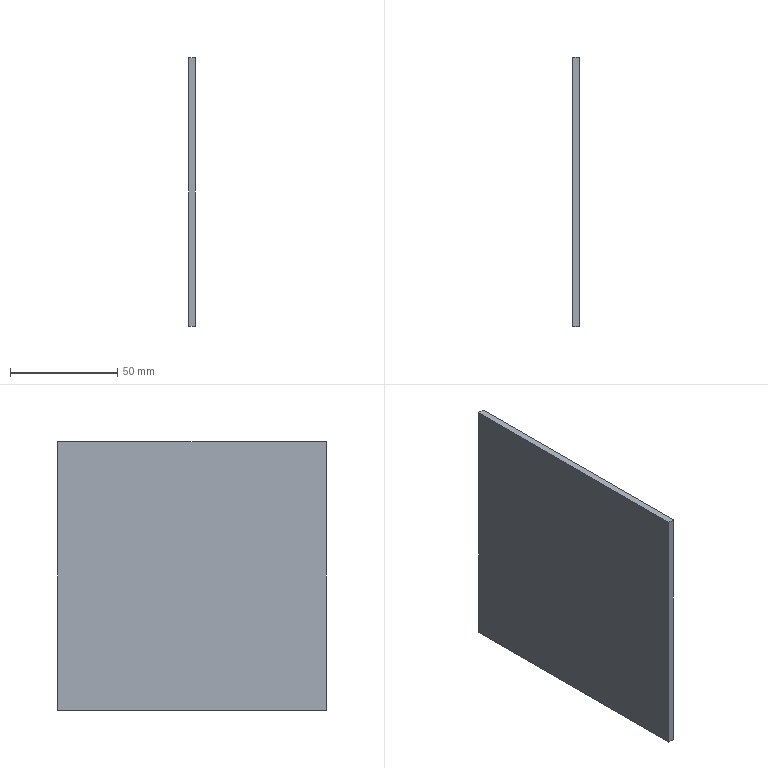Part | NX | features DATUM_CSYS 2, EXTRUDE 1, SKETCH 1 | 1 solid | 6 faces | box 3 x 125.6 x 125.6 mm | volume 47326 mm3 | plane 6
STEP:
#1=CARTESIAN_POINT('',(0.,0.,125.6));
#2=VERTEX_POINT('',#1);
#3=CARTESIAN_POINT('',(0.,0.,0.));
#4=VERTEX_POINT('',#3);
#5=CARTESIAN_POINT('',(0.,0.,125.6));
#6=DIRECTION('',(0.,0.,-1.));
#7=VECTOR('',#6,1000.);
#8=LINE('',#5,#7);
#9=EDGE_CURVE('',#2,#4,#8,.T.);
#10=ORIENTED_EDGE('',*,*,#9,.T.);
#11=CARTESIAN_POINT('',(3.,0.,0.));
#12=VERTEX_POINT('',#11);
#13=CARTESIAN_POINT('',(3.,0.,0.));
#14=DIRECTION('',(-1.,0.,0.));
#15=VECTOR('',#14,1000.);
#16=LINE('',#13,#15);
#17=EDGE_CURVE('',#12,#4,#16,.T.);
#18=ORIENTED_EDGE('',*,*,#17,.F.);
#19=CARTESIAN_POINT('',(3.,0.,125.6));
#20=VERTEX_POINT('',#19);
#21=CARTESIAN_POINT('',(3.,0.,125.6));
#22=DIRECTION('',(0.,0.,-1.));
#23=VECTOR('',#22,1000.);
#24=LINE('',#21,#23);
#25=EDGE_CURVE('',#20,#12,#24,.T.);
#26=ORIENTED_EDGE('',*,*,#25,.F.);
#27=CARTESIAN_POINT('',(3.,0.,125.6));
#28=DIRECTION('',(-1.,0.,0.));
#29=VECTOR('',#28,1000.);
#30=LINE('',#27,#29);
#31=EDGE_CURVE('',#20,#2,#30,.T.);
#32=ORIENTED_EDGE('',*,*,#31,.T.);
#33=EDGE_LOOP('',(#10,#18,#26,#32));
#34=FACE_BOUND('',#33,.T.);
#35=CARTESIAN_POINT('',(3.,0.,125.6));
#36=DIRECTION('',(0.,1.,0.));
#37=DIRECTION('',(0.,0.,1.));
#38=AXIS2_PLACEMENT_3D('',#35,#36,#37);
#39=PLANE('',#38);
#40=ADVANCED_FACE('',(#34),#39,.F.);
#41=CARTESIAN_POINT('',(0.,125.6,0.));
#42=VERTEX_POINT('',#41);
#43=CARTESIAN_POINT('',(0.,0.,0.));
#44=DIRECTION('',(0.,1.,0.));
#45=VECTOR('',#44,1000.);
#46=LINE('',#43,#45);
#47=EDGE_CURVE('',#4,#42,#46,.T.);
#48=ORIENTED_EDGE('',*,*,#47,.T.);
#49=CARTESIAN_POINT('',(3.,125.6,0.));
#50=VERTEX_POINT('',#49);
#51=CARTESIAN_POINT('',(3.,125.6,0.));
#52=DIRECTION('',(-1.,0.,0.));
#53=VECTOR('',#52,1000.);
#54=LINE('',#51,#53);
#55=EDGE_CURVE('',#50,#42,#54,.T.);
#56=ORIENTED_EDGE('',*,*,#55,.F.);
#57=CARTESIAN_POINT('',(3.,0.,0.));
#58=DIRECTION('',(0.,1.,0.));
#59=VECTOR('',#58,1000.);
#60=LINE('',#57,#59);
#61=EDGE_CURVE('',#12,#50,#60,.T.);
#62=ORIENTED_EDGE('',*,*,#61,.F.);
#63=ORIENTED_EDGE('',*,*,#17,.T.);
#64=EDGE_LOOP('',(#48,#56,#62,#63));
#65=FACE_BOUND('',#64,.T.);
#66=CARTESIAN_POINT('',(3.,0.,0.));
#67=DIRECTION('',(0.,0.,1.));
#68=DIRECTION('',(1.,0.,0.));
#69=AXIS2_PLACEMENT_3D('',#66,#67,#68);
#70=PLANE('',#69);
#71=ADVANCED_FACE('',(#65),#70,.F.);
#72=CARTESIAN_POINT('',(0.,125.6,125.6));
#73=VERTEX_POINT('',#72);
#74=CARTESIAN_POINT('',(0.,125.6,0.));
#75=DIRECTION('',(0.,0.,1.));
#76=VECTOR('',#75,1000.);
#77=LINE('',#74,#76);
#78=EDGE_CURVE('',#42,#73,#77,.T.);
#79=ORIENTED_EDGE('',*,*,#78,.T.);
#80=CARTESIAN_POINT('',(3.,125.6,125.6));
#81=VERTEX_POINT('',#80);
#82=CARTESIAN_POINT('',(3.,125.6,125.6));
#83=DIRECTION('',(-1.,0.,0.));
#84=VECTOR('',#83,1000.);
#85=LINE('',#82,#84);
#86=EDGE_CURVE('',#81,#73,#85,.T.);
#87=ORIENTED_EDGE('',*,*,#86,.F.);
#88=CARTESIAN_POINT('',(3.,125.6,0.));
#89=DIRECTION('',(0.,0.,1.));
#90=VECTOR('',#89,1000.);
#91=LINE('',#88,#90);
#92=EDGE_CURVE('',#50,#81,#91,.T.);
#93=ORIENTED_EDGE('',*,*,#92,.F.);
#94=ORIENTED_EDGE('',*,*,#55,.T.);
#95=EDGE_LOOP('',(#79,#87,#93,#94));
#96=FACE_BOUND('',#95,.T.);
#97=CARTESIAN_POINT('',(3.,125.6,0.));
#98=DIRECTION('',(0.,-1.,0.));
#99=DIRECTION('',(0.,0.,-1.));
#100=AXIS2_PLACEMENT_3D('',#97,#98,#99);
#101=PLANE('',#100);
#102=ADVANCED_FACE('',(#96),#101,.F.);
#103=CARTESIAN_POINT('',(0.,125.6,125.6));
#104=DIRECTION('',(0.,-1.,0.));
#105=VECTOR('',#104,1000.);
#106=LINE('',#103,#105);
#107=EDGE_CURVE('',#73,#2,#106,.T.);
#108=ORIENTED_EDGE('',*,*,#107,.T.);
#109=ORIENTED_EDGE('',*,*,#31,.F.);
#110=CARTESIAN_POINT('',(3.,125.6,125.6));
#111=DIRECTION('',(0.,-1.,0.));
#112=VECTOR('',#111,1000.);
#113=LINE('',#110,#112);
#114=EDGE_CURVE('',#81,#20,#113,.T.);
#115=ORIENTED_EDGE('',*,*,#114,.F.);
#116=ORIENTED_EDGE('',*,*,#86,.T.);
#117=EDGE_LOOP('',(#108,#109,#115,#116));
#118=FACE_BOUND('',#117,.T.);
#119=CARTESIAN_POINT('',(3.,125.6,125.6));
#120=DIRECTION('',(0.,0.,-1.));
#121=DIRECTION('',(0.,1.,0.));
#122=AXIS2_PLACEMENT_3D('',#119,#120,#121);
#123=PLANE('',#122);
#124=ADVANCED_FACE('',(#118),#123,.F.);
#125=ORIENTED_EDGE('',*,*,#25,.T.);
#126=ORIENTED_EDGE('',*,*,#61,.T.);
#127=ORIENTED_EDGE('',*,*,#92,.T.);
#128=ORIENTED_EDGE('',*,*,#114,.T.);
#129=EDGE_LOOP('',(#125,#126,#127,#128));
#130=FACE_BOUND('',#129,.T.);
#131=CARTESIAN_POINT('',(3.,0.,0.));
#132=DIRECTION('',(1.,0.,0.));
#133=DIRECTION('',(0.,0.,-1.));
#134=AXIS2_PLACEMENT_3D('',#131,#132,#133);
#135=PLANE('',#134);
#136=ADVANCED_FACE('',(#130),#135,.T.);
#137=ORIENTED_EDGE('',*,*,#9,.F.);
#138=ORIENTED_EDGE('',*,*,#107,.F.);
#139=ORIENTED_EDGE('',*,*,#78,.F.);
#140=ORIENTED_EDGE('',*,*,#47,.F.);
#141=EDGE_LOOP('',(#137,#138,#139,#140));
#142=FACE_BOUND('',#141,.T.);
#143=CARTESIAN_POINT('',(0.,0.,0.));
#144=DIRECTION('',(1.,0.,0.));
#145=DIRECTION('',(0.,0.,-1.));
#146=AXIS2_PLACEMENT_3D('',#143,#144,#145);
#147=PLANE('',#146);
#148=ADVANCED_FACE('',(#142),#147,.F.);
#149=CLOSED_SHELL('',(#40,#71,#102,#124,#136,#148));
#150=MANIFOLD_SOLID_BREP('',#149);
#151=(LENGTH_UNIT()NAMED_UNIT(*)SI_UNIT(.MILLI.,.METRE.));
#152=UNCERTAINTY_MEASURE_WITH_UNIT(LENGTH_MEASURE(0.00001),#151,'','');
#153=(NAMED_UNIT(*)PLANE_ANGLE_UNIT()SI_UNIT($,.RADIAN.));
#154=(NAMED_UNIT(*)SI_UNIT($,.STERADIAN.)SOLID_ANGLE_UNIT());
#155=(GEOMETRIC_REPRESENTATION_CONTEXT(3)GLOBAL_UNCERTAINTY_ASSIGNED_CONTEXT((#152))GLOBAL_UNIT_ASSIGNED_CONTEXT((#151,#153,#154))REPRESENTATION_CONTEXT('',''));
#156=ADVANCED_BREP_SHAPE_REPRESENTATION('',(#150),#155);